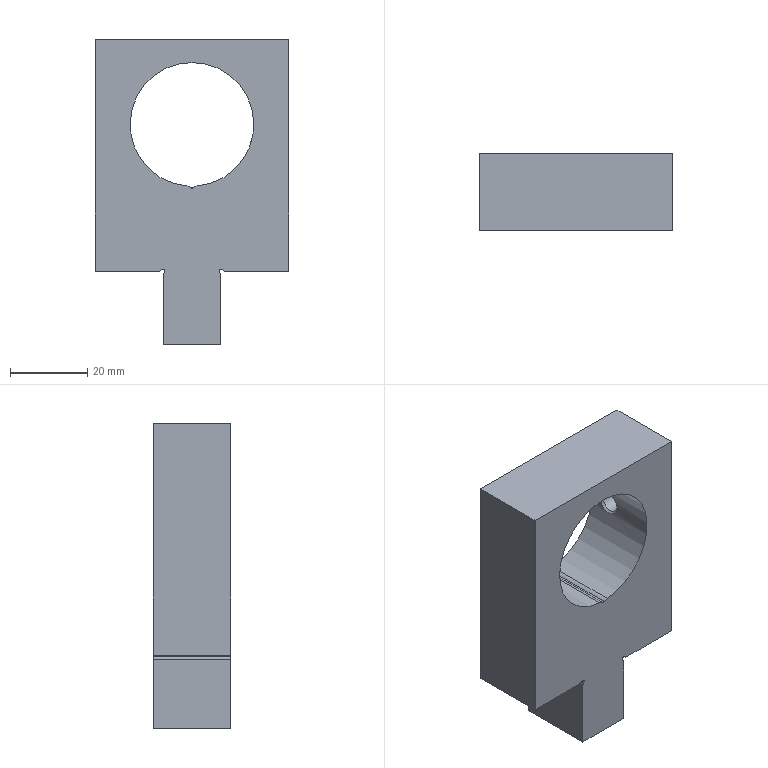Part | STEP file | 冲床-300配套压波_id890_x_t | 1 solid | 23 faces | box 50 x 20 x 79 mm | volume 49384 mm3 | cylinder 11 | plane 10 | spline 1 | cone 1 | commonest cylinder face diameters 2 x4 1 x3 4 x2 5 x1 32.01 x1
STEP:
#1=CARTESIAN_POINT('',(1916.413,80.,42.057));
#2=VERTEX_POINT('',#1);
#3=CARTESIAN_POINT('',(1913.587,80.,42.057));
#4=VERTEX_POINT('',#3);
#5=CARTESIAN_POINT('',(1915.,80.,58.));
#6=DIRECTION('',(0.,-1.,0.));
#7=DIRECTION('',(0.,0.,1.));
#8=AXIS2_PLACEMENT_3D('',#5,#6,#7);
#9=CIRCLE('',#8,16.005);
#10=EDGE_CURVE('',#2,#4,#9,.T.);
#11=ORIENTED_EDGE('',*,*,#10,.F.);
#12=CARTESIAN_POINT('',(1915.318,80.,41.609));
#13=VERTEX_POINT('',#12);
#14=CARTESIAN_POINT('',(1916.589,80.,40.065));
#15=DIRECTION('',(0.,-1.,0.));
#16=DIRECTION('',(0.,0.,1.));
#17=AXIS2_PLACEMENT_3D('',#14,#15,#16);
#18=CIRCLE('',#17,2.);
#19=EDGE_CURVE('',#2,#13,#18,.T.);
#20=ORIENTED_EDGE('',*,*,#19,.T.);
#21=CARTESIAN_POINT('',(1914.682,80.,41.609));
#22=VERTEX_POINT('',#21);
#23=CARTESIAN_POINT('',(1915.,80.,41.995));
#24=DIRECTION('',(0.,-1.,0.));
#25=DIRECTION('',(1.,0.,0.));
#26=AXIS2_PLACEMENT_3D('',#23,#24,#25);
#27=CIRCLE('',#26,0.5);
#28=EDGE_CURVE('',#22,#13,#27,.T.);
#29=ORIENTED_EDGE('',*,*,#28,.F.);
#30=CARTESIAN_POINT('',(1913.411,80.,40.065));
#31=DIRECTION('',(0.,-1.,0.));
#32=DIRECTION('',(0.,0.,1.));
#33=AXIS2_PLACEMENT_3D('',#30,#31,#32);
#34=CIRCLE('',#33,2.);
#35=EDGE_CURVE('',#22,#4,#34,.T.);
#36=ORIENTED_EDGE('',*,*,#35,.T.);
#37=EDGE_LOOP('',(#11,#20,#29,#36));
#38=FACE_BOUND('',#37,.T.);
#39=CARTESIAN_POINT('',(1890.,80.,80.));
#40=VERTEX_POINT('',#39);
#41=CARTESIAN_POINT('',(1940.,80.,80.));
#42=VERTEX_POINT('',#41);
#43=CARTESIAN_POINT('',(1940.,80.,80.));
#44=DIRECTION('',(1.,0.,0.));
#45=VECTOR('',#44,1.);
#46=LINE('',#43,#45);
#47=EDGE_CURVE('',#40,#42,#46,.T.);
#48=ORIENTED_EDGE('',*,*,#47,.F.);
#49=CARTESIAN_POINT('',(1890.,80.,20.));
#50=VERTEX_POINT('',#49);
#51=CARTESIAN_POINT('',(1890.,80.,20.));
#52=DIRECTION('',(0.,0.,1.));
#53=VECTOR('',#52,1.);
#54=LINE('',#51,#53);
#55=EDGE_CURVE('',#50,#40,#54,.T.);
#56=ORIENTED_EDGE('',*,*,#55,.F.);
#57=CARTESIAN_POINT('',(1906.382,80.,20.));
#58=VERTEX_POINT('',#57);
#59=CARTESIAN_POINT('',(1940.,80.,20.));
#60=DIRECTION('',(1.,0.,0.));
#61=VECTOR('',#60,1.);
#62=LINE('',#59,#61);
#63=EDGE_CURVE('',#50,#58,#62,.T.);
#64=ORIENTED_EDGE('',*,*,#63,.T.);
#65=CARTESIAN_POINT('',(1907.127,80.,20.333));
#66=VERTEX_POINT('',#65);
#67=CARTESIAN_POINT('',(1906.382,80.,21.));
#68=DIRECTION('',(0.,-1.,0.));
#69=DIRECTION('',(0.,0.,-1.));
#70=AXIS2_PLACEMENT_3D('',#67,#68,#69);
#71=CIRCLE('',#70,1.);
#72=EDGE_CURVE('',#58,#66,#71,.T.);
#73=ORIENTED_EDGE('',*,*,#72,.T.);
#74=CARTESIAN_POINT('',(1907.833,80.,19.627));
#75=VERTEX_POINT('',#74);
#76=CARTESIAN_POINT('',(1907.5,80.,20.));
#77=DIRECTION('',(0.,-1.,0.));
#78=DIRECTION('',(-1.,0.,0.));
#79=AXIS2_PLACEMENT_3D('',#76,#77,#78);
#80=CIRCLE('',#79,0.5);
#81=EDGE_CURVE('',#75,#66,#80,.T.);
#82=ORIENTED_EDGE('',*,*,#81,.F.);
#83=CARTESIAN_POINT('',(1907.5,80.,18.882));
#84=VERTEX_POINT('',#83);
#85=CARTESIAN_POINT('',(1908.5,80.,18.882));
#86=DIRECTION('',(0.,-1.,0.));
#87=DIRECTION('',(0.,0.,-1.));
#88=AXIS2_PLACEMENT_3D('',#85,#86,#87);
#89=CIRCLE('',#88,1.);
#90=EDGE_CURVE('',#75,#84,#89,.T.);
#91=ORIENTED_EDGE('',*,*,#90,.T.);
#92=CARTESIAN_POINT('',(1907.5,80.,1.));
#93=VERTEX_POINT('',#92);
#94=CARTESIAN_POINT('',(1907.5,80.,20.));
#95=DIRECTION('',(0.,0.,-1.));
#96=VECTOR('',#95,1.);
#97=LINE('',#94,#96);
#98=EDGE_CURVE('',#84,#93,#97,.T.);
#99=ORIENTED_EDGE('',*,*,#98,.T.);
#100=CARTESIAN_POINT('',(1922.5,80.,1.));
#101=VERTEX_POINT('',#100);
#102=CARTESIAN_POINT('',(1940.,80.,1.));
#103=DIRECTION('',(1.,0.,0.));
#104=VECTOR('',#103,1.);
#105=LINE('',#102,#104);
#106=EDGE_CURVE('',#93,#101,#105,.T.);
#107=ORIENTED_EDGE('',*,*,#106,.T.);
#108=CARTESIAN_POINT('',(1922.5,80.,18.882));
#109=VERTEX_POINT('',#108);
#110=CARTESIAN_POINT('',(1922.5,80.,-62.5));
#111=DIRECTION('',(0.,0.,1.));
#112=VECTOR('',#111,1.);
#113=LINE('',#110,#112);
#114=EDGE_CURVE('',#101,#109,#113,.T.);
#115=ORIENTED_EDGE('',*,*,#114,.T.);
#116=CARTESIAN_POINT('',(1922.167,80.,19.627));
#117=VERTEX_POINT('',#116);
#118=CARTESIAN_POINT('',(1921.5,80.,18.882));
#119=DIRECTION('',(0.,-1.,0.));
#120=DIRECTION('',(0.,0.,-1.));
#121=AXIS2_PLACEMENT_3D('',#118,#119,#120);
#122=CIRCLE('',#121,1.);
#123=EDGE_CURVE('',#109,#117,#122,.T.);
#124=ORIENTED_EDGE('',*,*,#123,.T.);
#125=CARTESIAN_POINT('',(1922.873,80.,20.333));
#126=VERTEX_POINT('',#125);
#127=CARTESIAN_POINT('',(1922.5,80.,20.));
#128=DIRECTION('',(0.,-1.,0.));
#129=DIRECTION('',(1.,0.,0.));
#130=AXIS2_PLACEMENT_3D('',#127,#128,#129);
#131=CIRCLE('',#130,0.5);
#132=EDGE_CURVE('',#126,#117,#131,.T.);
#133=ORIENTED_EDGE('',*,*,#132,.F.);
#134=CARTESIAN_POINT('',(1923.618,80.,20.));
#135=VERTEX_POINT('',#134);
#136=CARTESIAN_POINT('',(1923.618,80.,21.));
#137=DIRECTION('',(0.,-1.,0.));
#138=DIRECTION('',(0.,0.,-1.));
#139=AXIS2_PLACEMENT_3D('',#136,#137,#138);
#140=CIRCLE('',#139,1.);
#141=EDGE_CURVE('',#126,#135,#140,.T.);
#142=ORIENTED_EDGE('',*,*,#141,.T.);
#143=CARTESIAN_POINT('',(1940.,80.,20.));
#144=VERTEX_POINT('',#143);
#145=CARTESIAN_POINT('',(1940.,80.,20.));
#146=DIRECTION('',(1.,0.,0.));
#147=VECTOR('',#146,1.);
#148=LINE('',#145,#147);
#149=EDGE_CURVE('',#135,#144,#148,.T.);
#150=ORIENTED_EDGE('',*,*,#149,.T.);
#151=CARTESIAN_POINT('',(1940.,80.,20.));
#152=DIRECTION('',(0.,0.,1.));
#153=VECTOR('',#152,1.);
#154=LINE('',#151,#153);
#155=EDGE_CURVE('',#144,#42,#154,.T.);
#156=ORIENTED_EDGE('',*,*,#155,.T.);
#157=EDGE_LOOP('',(#48,#56,#64,#73,#82,#91,#99,#107,#115,#124,#133,#142,#150,#156));
#158=FACE_BOUND('',#157,.T.);
#159=CARTESIAN_POINT('',(1940.,80.,20.));
#160=DIRECTION('',(0.,1.,0.));
#161=DIRECTION('',(0.,0.,-1.));
#162=AXIS2_PLACEMENT_3D('',#159,#160,#161);
#163=PLANE('',#162);
#164=ADVANCED_FACE('',(#38,#158),#163,.F.);
#165=CARTESIAN_POINT('',(1915.318,100.,41.609));
#166=VERTEX_POINT('',#165);
#167=CARTESIAN_POINT('',(1914.682,100.,41.609));
#168=VERTEX_POINT('',#167);
#169=CARTESIAN_POINT('',(1915.,100.,41.995));
#170=DIRECTION('',(0.,1.,0.));
#171=DIRECTION('',(1.,0.,0.));
#172=AXIS2_PLACEMENT_3D('',#169,#170,#171);
#173=CIRCLE('',#172,0.5);
#174=EDGE_CURVE('',#166,#168,#173,.T.);
#175=ORIENTED_EDGE('',*,*,#174,.F.);
#176=CARTESIAN_POINT('',(1916.413,100.,42.057));
#177=VERTEX_POINT('',#176);
#178=CARTESIAN_POINT('',(1916.589,100.,40.065));
#179=DIRECTION('',(0.,1.,0.));
#180=DIRECTION('',(0.,0.,-1.));
#181=AXIS2_PLACEMENT_3D('',#178,#179,#180);
#182=CIRCLE('',#181,2.);
#183=EDGE_CURVE('',#166,#177,#182,.T.);
#184=ORIENTED_EDGE('',*,*,#183,.T.);
#185=CARTESIAN_POINT('',(1913.587,100.,42.057));
#186=VERTEX_POINT('',#185);
#187=CARTESIAN_POINT('',(1915.,100.,58.));
#188=DIRECTION('',(0.,1.,0.));
#189=DIRECTION('',(0.,0.,-1.));
#190=AXIS2_PLACEMENT_3D('',#187,#188,#189);
#191=CIRCLE('',#190,16.005);
#192=EDGE_CURVE('',#186,#177,#191,.T.);
#193=ORIENTED_EDGE('',*,*,#192,.F.);
#194=CARTESIAN_POINT('',(1913.411,100.,40.065));
#195=DIRECTION('',(0.,1.,0.));
#196=DIRECTION('',(0.,0.,-1.));
#197=AXIS2_PLACEMENT_3D('',#194,#195,#196);
#198=CIRCLE('',#197,2.);
#199=EDGE_CURVE('',#186,#168,#198,.T.);
#200=ORIENTED_EDGE('',*,*,#199,.T.);
#201=EDGE_LOOP('',(#175,#184,#193,#200));
#202=FACE_BOUND('',#201,.T.);
#203=CARTESIAN_POINT('',(1940.,100.,80.));
#204=VERTEX_POINT('',#203);
#205=CARTESIAN_POINT('',(1890.,100.,80.));
#206=VERTEX_POINT('',#205);
#207=CARTESIAN_POINT('',(1940.,100.,80.));
#208=DIRECTION('',(-1.,0.,0.));
#209=VECTOR('',#208,1.);
#210=LINE('',#207,#209);
#211=EDGE_CURVE('',#204,#206,#210,.T.);
#212=ORIENTED_EDGE('',*,*,#211,.F.);
#213=CARTESIAN_POINT('',(1940.,100.,20.));
#214=VERTEX_POINT('',#213);
#215=CARTESIAN_POINT('',(1940.,100.,20.));
#216=DIRECTION('',(0.,0.,-1.));
#217=VECTOR('',#216,1.);
#218=LINE('',#215,#217);
#219=EDGE_CURVE('',#204,#214,#218,.T.);
#220=ORIENTED_EDGE('',*,*,#219,.T.);
#221=CARTESIAN_POINT('',(1923.618,100.,20.));
#222=VERTEX_POINT('',#221);
#223=CARTESIAN_POINT('',(1940.,100.,20.));
#224=DIRECTION('',(-1.,0.,0.));
#225=VECTOR('',#224,1.);
#226=LINE('',#223,#225);
#227=EDGE_CURVE('',#214,#222,#226,.T.);
#228=ORIENTED_EDGE('',*,*,#227,.T.);
#229=CARTESIAN_POINT('',(1922.873,100.,20.333));
#230=VERTEX_POINT('',#229);
#231=CARTESIAN_POINT('',(1923.618,100.,21.));
#232=DIRECTION('',(0.,1.,0.));
#233=DIRECTION('',(0.,0.,1.));
#234=AXIS2_PLACEMENT_3D('',#231,#232,#233);
#235=CIRCLE('',#234,1.);
#236=EDGE_CURVE('',#222,#230,#235,.T.);
#237=ORIENTED_EDGE('',*,*,#236,.T.);
#238=CARTESIAN_POINT('',(1922.167,100.,19.627));
#239=VERTEX_POINT('',#238);
#240=CARTESIAN_POINT('',(1922.5,100.,20.));
#241=DIRECTION('',(0.,1.,0.));
#242=DIRECTION('',(1.,0.,0.));
#243=AXIS2_PLACEMENT_3D('',#240,#241,#242);
#244=CIRCLE('',#243,0.5);
#245=EDGE_CURVE('',#239,#230,#244,.T.);
#246=ORIENTED_EDGE('',*,*,#245,.F.);
#247=CARTESIAN_POINT('',(1922.5,100.,18.882));
#248=VERTEX_POINT('',#247);
#249=CARTESIAN_POINT('',(1921.5,100.,18.882));
#250=DIRECTION('',(0.,1.,0.));
#251=DIRECTION('',(0.,0.,1.));
#252=AXIS2_PLACEMENT_3D('',#249,#250,#251);
#253=CIRCLE('',#252,1.);
#254=EDGE_CURVE('',#239,#248,#253,.T.);
#255=ORIENTED_EDGE('',*,*,#254,.T.);
#256=CARTESIAN_POINT('',(1922.5,100.,1.));
#257=VERTEX_POINT('',#256);
#258=CARTESIAN_POINT('',(1922.5,100.,20.));
#259=DIRECTION('',(0.,0.,-1.));
#260=VECTOR('',#259,1.);
#261=LINE('',#258,#260);
#262=EDGE_CURVE('',#248,#257,#261,.T.);
#263=ORIENTED_EDGE('',*,*,#262,.T.);
#264=CARTESIAN_POINT('',(1907.5,100.,1.));
#265=VERTEX_POINT('',#264);
#266=CARTESIAN_POINT('',(1940.,100.,1.));
#267=DIRECTION('',(-1.,0.,0.));
#268=VECTOR('',#267,1.);
#269=LINE('',#266,#268);
#270=EDGE_CURVE('',#257,#265,#269,.T.);
#271=ORIENTED_EDGE('',*,*,#270,.T.);
#272=CARTESIAN_POINT('',(1907.5,100.,18.882));
#273=VERTEX_POINT('',#272);
#274=CARTESIAN_POINT('',(1907.5,100.,-62.5));
#275=DIRECTION('',(0.,0.,1.));
#276=VECTOR('',#275,1.);
#277=LINE('',#274,#276);
#278=EDGE_CURVE('',#265,#273,#277,.T.);
#279=ORIENTED_EDGE('',*,*,#278,.T.);
#280=CARTESIAN_POINT('',(1907.833,100.,19.627));
#281=VERTEX_POINT('',#280);
#282=CARTESIAN_POINT('',(1908.5,100.,18.882));
#283=DIRECTION('',(0.,1.,0.));
#284=DIRECTION('',(0.,0.,1.));
#285=AXIS2_PLACEMENT_3D('',#282,#283,#284);
#286=CIRCLE('',#285,1.);
#287=EDGE_CURVE('',#273,#281,#286,.T.);
#288=ORIENTED_EDGE('',*,*,#287,.T.);
#289=CARTESIAN_POINT('',(1907.127,100.,20.333));
#290=VERTEX_POINT('',#289);
#291=CARTESIAN_POINT('',(1907.5,100.,20.));
#292=DIRECTION('',(0.,1.,0.));
#293=DIRECTION('',(-1.,0.,0.));
#294=AXIS2_PLACEMENT_3D('',#291,#292,#293);
#295=CIRCLE('',#294,0.5);
#296=EDGE_CURVE('',#290,#281,#295,.T.);
#297=ORIENTED_EDGE('',*,*,#296,.F.);
#298=CARTESIAN_POINT('',(1906.382,100.,20.));
#299=VERTEX_POINT('',#298);
#300=CARTESIAN_POINT('',(1906.382,100.,21.));
#301=DIRECTION('',(0.,1.,0.));
#302=DIRECTION('',(0.,0.,1.));
#303=AXIS2_PLACEMENT_3D('',#300,#301,#302);
#304=CIRCLE('',#303,1.);
#305=EDGE_CURVE('',#290,#299,#304,.T.);
#306=ORIENTED_EDGE('',*,*,#305,.T.);
#307=CARTESIAN_POINT('',(1890.,100.,20.));
#308=VERTEX_POINT('',#307);
#309=CARTESIAN_POINT('',(1940.,100.,20.));
#310=DIRECTION('',(-1.,0.,0.));
#311=VECTOR('',#310,1.);
#312=LINE('',#309,#311);
#313=EDGE_CURVE('',#299,#308,#312,.T.);
#314=ORIENTED_EDGE('',*,*,#313,.T.);
#315=CARTESIAN_POINT('',(1890.,100.,20.));
#316=DIRECTION('',(0.,0.,-1.));
#317=VECTOR('',#316,1.);
#318=LINE('',#315,#317);
#319=EDGE_CURVE('',#206,#308,#318,.T.);
#320=ORIENTED_EDGE('',*,*,#319,.F.);
#321=EDGE_LOOP('',(#212,#220,#228,#237,#246,#255,#263,#271,#279,#288,#297,#306,#314,#320));
#322=FACE_BOUND('',#321,.T.);
#323=CARTESIAN_POINT('',(1940.,100.,20.));
#324=DIRECTION('',(0.,-1.,0.));
#325=DIRECTION('',(0.,0.,1.));
#326=AXIS2_PLACEMENT_3D('',#323,#324,#325);
#327=PLANE('',#326);
#328=ADVANCED_FACE('',(#202,#322),#327,.F.);
#329=CARTESIAN_POINT('',(1890.,80.,80.));
#330=DIRECTION('',(0.,-1.,0.));
#331=VECTOR('',#330,1.);
#332=LINE('',#329,#331);
#333=EDGE_CURVE('',#206,#40,#332,.T.);
#334=ORIENTED_EDGE('',*,*,#333,.F.);
#335=ORIENTED_EDGE('',*,*,#319,.T.);
#336=CARTESIAN_POINT('',(1890.,-80.,20.));
#337=DIRECTION('',(0.,-1.,0.));
#338=VECTOR('',#337,1.);
#339=LINE('',#336,#338);
#340=EDGE_CURVE('',#308,#50,#339,.T.);
#341=ORIENTED_EDGE('',*,*,#340,.T.);
#342=ORIENTED_EDGE('',*,*,#55,.T.);
#343=EDGE_LOOP('',(#334,#335,#341,#342));
#344=FACE_OUTER_BOUND('',#343,.T.);
#345=CARTESIAN_POINT('',(1890.,80.,20.));
#346=DIRECTION('',(1.,0.,0.));
#347=DIRECTION('',(0.,0.,-1.));
#348=AXIS2_PLACEMENT_3D('',#345,#346,#347);
#349=PLANE('',#348);
#350=ADVANCED_FACE('',(#344),#349,.F.);
#351=CARTESIAN_POINT('',(1940.,94.,61.));
#352=VERTEX_POINT('',#351);
#353=CARTESIAN_POINT('',(1940.,94.,58.));
#354=DIRECTION('',(-1.,0.,0.));
#355=DIRECTION('',(0.,0.,1.));
#356=AXIS2_PLACEMENT_3D('',#353,#354,#355);
#357=CIRCLE('',#356,3.);
#358=EDGE_CURVE('',#352,#352,#357,.T.);
#359=ORIENTED_EDGE('',*,*,#358,.T.);
#360=EDGE_LOOP('',(#359));
#361=FACE_BOUND('',#360,.T.);
#362=CARTESIAN_POINT('',(1940.,150.,80.));
#363=DIRECTION('',(0.,1.,0.));
#364=VECTOR('',#363,1.);
#365=LINE('',#362,#364);
#366=EDGE_CURVE('',#42,#204,#365,.T.);
#367=ORIENTED_EDGE('',*,*,#366,.F.);
#368=ORIENTED_EDGE('',*,*,#155,.F.);
#369=CARTESIAN_POINT('',(1940.,-150.,20.));
#370=DIRECTION('',(0.,1.,0.));
#371=VECTOR('',#370,1.);
#372=LINE('',#369,#371);
#373=EDGE_CURVE('',#144,#214,#372,.T.);
#374=ORIENTED_EDGE('',*,*,#373,.T.);
#375=ORIENTED_EDGE('',*,*,#219,.F.);
#376=EDGE_LOOP('',(#367,#368,#374,#375));
#377=FACE_BOUND('',#376,.T.);
#378=CARTESIAN_POINT('',(1940.,150.,20.));
#379=DIRECTION('',(-1.,0.,0.));
#380=DIRECTION('',(0.,0.,1.));
#381=AXIS2_PLACEMENT_3D('',#378,#379,#380);
#382=PLANE('',#381);
#383=ADVANCED_FACE('',(#361,#377),#382,.F.);
#384=ORIENTED_EDGE('',*,*,#28,.T.);
#385=CARTESIAN_POINT('',(1915.318,80.,41.609));
#386=DIRECTION('',(0.,1.,0.));
#387=VECTOR('',#386,1.);
#388=LINE('',#385,#387);
#389=EDGE_CURVE('',#13,#166,#388,.T.);
#390=ORIENTED_EDGE('',*,*,#389,.T.);
#391=ORIENTED_EDGE('',*,*,#174,.T.);
#392=CARTESIAN_POINT('',(1914.682,80.,41.609));
#393=DIRECTION('',(0.,-1.,0.));
#394=VECTOR('',#393,1.);
#395=LINE('',#392,#394);
#396=EDGE_CURVE('',#168,#22,#395,.T.);
#397=ORIENTED_EDGE('',*,*,#396,.T.);
#398=EDGE_LOOP('',(#384,#390,#391,#397));
#399=FACE_OUTER_BOUND('',#398,.T.);
#400=CARTESIAN_POINT('',(1915.,80.,41.995));
#401=DIRECTION('',(0.,1.,0.));
#402=DIRECTION('',(0.,0.,1.));
#403=AXIS2_PLACEMENT_3D('',#400,#401,#402);
#404=CYLINDRICAL_SURFACE('',#403,0.5);
#405=ADVANCED_FACE('',(#399),#404,.F.);
#406=ORIENTED_EDGE('',*,*,#183,.F.);
#407=ORIENTED_EDGE('',*,*,#389,.F.);
#408=ORIENTED_EDGE('',*,*,#19,.F.);
#409=CARTESIAN_POINT('',(1916.413,105.,42.057));
#410=DIRECTION('',(0.,-1.,0.));
#411=VECTOR('',#410,1.);
#412=LINE('',#409,#411);
#413=EDGE_CURVE('',#177,#2,#412,.T.);
#414=ORIENTED_EDGE('',*,*,#413,.F.);
#415=EDGE_LOOP('',(#406,#407,#408,#414));
#416=FACE_OUTER_BOUND('',#415,.T.);
#417=CARTESIAN_POINT('',(1916.589,80.,40.065));
#418=DIRECTION('',(0.,-1.,0.));
#419=DIRECTION('',(0.,0.,-1.));
#420=AXIS2_PLACEMENT_3D('',#417,#418,#419);
#421=CYLINDRICAL_SURFACE('',#420,2.);
#422=ADVANCED_FACE('',(#416),#421,.T.);
#423=CARTESIAN_POINT('',(1931.303,94.,60.5));
#424=VERTEX_POINT('',#423);
#425=CARTESIAN_POINT('',(1931.303,94.,60.5));
#426=CARTESIAN_POINT('',(1931.303,94.488,60.5));
#427=CARTESIAN_POINT('',(1931.351,95.187,60.349));
#428=CARTESIAN_POINT('',(1931.445,95.768,59.768));
#429=CARTESIAN_POINT('',(1931.539,96.349,59.187));
#430=CARTESIAN_POINT('',(1931.585,96.5,58.495));
#431=CARTESIAN_POINT('',(1931.585,96.5,58.001));
#432=CARTESIAN_POINT('',(1931.585,96.5,57.508));
#433=CARTESIAN_POINT('',(1931.538,96.344,56.809));
#434=CARTESIAN_POINT('',(1931.445,95.768,56.233));
#435=CARTESIAN_POINT('',(1931.351,95.192,55.656));
#436=CARTESIAN_POINT('',(1931.303,94.486,55.5));
#437=CARTESIAN_POINT('',(1931.303,94.,55.5));
#438=CARTESIAN_POINT('',(1931.303,93.513,55.5));
#439=CARTESIAN_POINT('',(1931.351,92.813,55.651));
#440=CARTESIAN_POINT('',(1931.445,92.231,56.233));
#441=CARTESIAN_POINT('',(1931.539,91.65,56.815));
#442=CARTESIAN_POINT('',(1931.585,91.5,57.507));
#443=CARTESIAN_POINT('',(1931.585,91.5,58.001));
#444=CARTESIAN_POINT('',(1931.585,91.5,58.496));
#445=CARTESIAN_POINT('',(1931.538,91.656,59.192));
#446=CARTESIAN_POINT('',(1931.445,92.232,59.768));
#447=CARTESIAN_POINT('',(1931.351,92.808,60.343));
#448=CARTESIAN_POINT('',(1931.303,93.512,60.5));
#449=CARTESIAN_POINT('',(1931.303,94.,60.5));
#450=B_SPLINE_CURVE_WITH_KNOTS('',3,(#425,#426,#427,#428,#429,#430,#431,#432,#433,#434,#435,#436,#437,#438,#439,#440,#441,#442,#443,#444,#445,#446,#447,#448,#449),.UNSPECIFIED.,.T.,.F.,(1,3,3,3,3,3,3,3,3,3,1),(-0.125,0.,0.125,0.25,0.375,0.5,0.625,0.75,0.875,1.,1.125),.UNSPECIFIED.);
#451=EDGE_CURVE('',#424,#424,#450,.T.);
#452=ORIENTED_EDGE('',*,*,#451,.T.);
#453=EDGE_LOOP('',(#452));
#454=FACE_BOUND('',#453,.T.);
#455=CARTESIAN_POINT('',(1939.5,94.,60.5));
#456=VERTEX_POINT('',#455);
#457=CARTESIAN_POINT('',(1939.5,94.,58.));
#458=DIRECTION('',(1.,0.,0.));
#459=DIRECTION('',(0.,0.,1.));
#460=AXIS2_PLACEMENT_3D('',#457,#458,#459);
#461=CIRCLE('',#460,2.5);
#462=EDGE_CURVE('',#456,#456,#461,.T.);
#463=ORIENTED_EDGE('',*,*,#462,.T.);
#464=EDGE_LOOP('',(#463));
#465=FACE_BOUND('',#464,.T.);
#466=CARTESIAN_POINT('',(1940.,94.,58.));
#467=DIRECTION('',(-1.,0.,0.));
#468=DIRECTION('',(0.,0.,1.));
#469=AXIS2_PLACEMENT_3D('',#466,#467,#468);
#470=CYLINDRICAL_SURFACE('',#469,2.5);
#471=ADVANCED_FACE('',(#454,#465),#470,.F.);
#472=CARTESIAN_POINT('',(1930.734,94.,55.068));
#473=VERTEX_POINT('',#472);
#474=CARTESIAN_POINT('',(1930.734,94.,55.068));
#475=CARTESIAN_POINT('',(1930.734,94.344,55.068));
#476=CARTESIAN_POINT('',(1930.745,94.693,55.127));
#477=CARTESIAN_POINT('',(1930.765,95.018,55.238));
#478=CARTESIAN_POINT('',(1930.785,95.343,55.35));
#479=CARTESIAN_POINT('',(1930.813,95.654,55.519));
#480=CARTESIAN_POINT('',(1930.843,95.924,55.731));
#481=CARTESIAN_POINT('',(1930.874,96.197,55.945));
#482=CARTESIAN_POINT('',(1930.908,96.434,56.212));
#483=CARTESIAN_POINT('',(1930.935,96.614,56.509));
#484=CARTESIAN_POINT('',(1930.962,96.783,56.788));
#485=CARTESIAN_POINT('',(1930.983,96.908,57.1));
#486=CARTESIAN_POINT('',(1930.994,96.977,57.42));
#487=CARTESIAN_POINT('',(1931.006,97.046,57.742));
#488=CARTESIAN_POINT('',(1931.008,97.058,58.082));
#489=CARTESIAN_POINT('',(1931.,97.009,58.408));
#490=CARTESIAN_POINT('',(1930.992,96.964,58.709));
#491=CARTESIAN_POINT('',(1930.976,96.869,59.005));
#492=CARTESIAN_POINT('',(1930.954,96.733,59.277));
#493=CARTESIAN_POINT('',(1930.931,96.589,59.565));
#494=CARTESIAN_POINT('',(1930.901,96.395,59.833));
#495=CARTESIAN_POINT('',(1930.872,96.165,60.058));
#496=CARTESIAN_POINT('',(1930.843,95.933,60.285));
#497=CARTESIAN_POINT('',(1930.813,95.659,60.475));
#498=CARTESIAN_POINT('',(1930.79,95.366,60.617));
#499=CARTESIAN_POINT('',(1930.765,95.059,60.766));
#500=CARTESIAN_POINT('',(1930.746,94.722,60.866));
#501=CARTESIAN_POINT('',(1930.739,94.383,60.908));
#502=CARTESIAN_POINT('',(1930.737,94.297,60.919));
#503=CARTESIAN_POINT('',(1930.735,94.211,60.926));
#504=CARTESIAN_POINT('',(1930.735,94.125,60.93));
#505=CARTESIAN_POINT('',(1930.734,94.039,60.933));
#506=CARTESIAN_POINT('',(1930.734,93.953,60.933));
#507=CARTESIAN_POINT('',(1930.735,93.867,60.929));
#508=CARTESIAN_POINT('',(1930.737,93.524,60.914));
#509=CARTESIAN_POINT('',(1930.751,93.179,60.841));
#510=CARTESIAN_POINT('',(1930.773,92.86,60.716));
#511=CARTESIAN_POINT('',(1930.794,92.541,60.591));
#512=CARTESIAN_POINT('',(1930.824,92.239,60.412));
#513=CARTESIAN_POINT('',(1930.854,91.979,60.19));
#514=CARTESIAN_POINT('',(1930.886,91.715,59.965));
#515=CARTESIAN_POINT('',(1930.919,91.49,59.687));
#516=CARTESIAN_POINT('',(1930.945,91.323,59.383));
#517=CARTESIAN_POINT('',(1930.97,91.166,59.098));
#518=CARTESIAN_POINT('',(1930.989,91.054,58.782));
#519=CARTESIAN_POINT('',(1930.998,90.999,58.461));
#520=CARTESIAN_POINT('',(1931.008,90.945,58.139));
#521=CARTESIAN_POINT('',(1931.007,90.949,57.802));
#522=CARTESIAN_POINT('',(1930.997,91.01,57.482));
#523=CARTESIAN_POINT('',(1930.987,91.067,57.184));
#524=CARTESIAN_POINT('',(1930.969,91.173,56.892));
#525=CARTESIAN_POINT('',(1930.946,91.318,56.626));
#526=CARTESIAN_POINT('',(1930.921,91.474,56.34));
#527=CARTESIAN_POINT('',(1930.891,91.681,56.077));
#528=CARTESIAN_POINT('',(1930.861,91.923,55.859));
#529=CARTESIAN_POINT('',(1930.832,92.165,55.642));
#530=CARTESIAN_POINT('',(1930.803,92.445,55.463));
#531=CARTESIAN_POINT('',(1930.781,92.742,55.332));
#532=CARTESIAN_POINT('',(1930.758,93.057,55.194));
#533=CARTESIAN_POINT('',(1930.741,93.4,55.107));
#534=CARTESIAN_POINT('',(1930.736,93.744,55.078));
#535=CARTESIAN_POINT('',(1930.735,93.829,55.071));
#536=CARTESIAN_POINT('',(1930.734,93.914,55.068));
#537=CARTESIAN_POINT('',(1930.734,94.,55.068));
#538=B_SPLINE_CURVE_WITH_KNOTS('',3,(#474,#475,#476,#477,#478,#479,#480,#481,#482,#483,#484,#485,#486,#487,#488,#489,#490,#491,#492,#493,#494,#495,#496,#497,#498,#499,#500,#501,#502,#503,#504,#505,#506,#507,#508,#509,#510,#511,#512,#513,#514,#515,#516,#517,#518,#519,#520,#521,#522,#523,#524,#525,#526,#527,#528,#529,#530,#531,#532,#533,#534,#535,#536,#537),.UNSPECIFIED.,.T.,.F.,(1,3,3,3,3,3,3,3,3,3,3,3,3,3,3,3,3,3,3,3,3,3,3,1),(-0.01354,0.,0.05524,0.1106,0.1666,0.2191,0.2721,0.3208,0.3727,0.4249,0.4798,0.4934,0.5071,0.5622,0.6172,0.6731,0.7255,0.7779,0.8265,0.879,0.9312,0.9865,1.,1.055),.UNSPECIFIED.);
#539=EDGE_CURVE('',#473,#473,#538,.T.);
#540=ORIENTED_EDGE('',*,*,#539,.F.);
#541=EDGE_LOOP('',(#540));
#542=FACE_BOUND('',#541,.T.);
#543=ORIENTED_EDGE('',*,*,#451,.F.);
#544=EDGE_LOOP('',(#543));
#545=FACE_BOUND('',#544,.T.);
#546=CARTESIAN_POINT('',(1931.303,94.657,60.5));
#547=CARTESIAN_POINT('',(1931.303,93.343,60.5));
#548=CARTESIAN_POINT('',(1931.37,92.694,60.229));
#549=CARTESIAN_POINT('',(1931.52,91.77,59.306));
#550=CARTESIAN_POINT('',(1931.585,91.5,58.658));
#551=CARTESIAN_POINT('',(1931.585,91.5,57.344));
#552=CARTESIAN_POINT('',(1931.52,91.769,56.696));
#553=CARTESIAN_POINT('',(1931.37,92.694,55.77));
#554=CARTESIAN_POINT('',(1931.303,93.34,55.5));
#555=CARTESIAN_POINT('',(1931.303,94.66,55.5));
#556=CARTESIAN_POINT('',(1931.37,95.306,55.77));
#557=CARTESIAN_POINT('',(1931.52,96.231,56.695));
#558=CARTESIAN_POINT('',(1931.585,96.5,57.345));
#559=CARTESIAN_POINT('',(1931.585,96.5,58.658));
#560=CARTESIAN_POINT('',(1931.52,96.23,59.306));
#561=CARTESIAN_POINT('',(1931.37,95.306,60.229));
#562=CARTESIAN_POINT('',(1931.303,94.657,60.5));
#563=CARTESIAN_POINT('',(1931.303,93.343,60.5));
#564=CARTESIAN_POINT('',(1930.728,94.801,60.937));
#565=CARTESIAN_POINT('',(1930.728,93.199,60.937));
#566=CARTESIAN_POINT('',(1930.792,92.41,60.619));
#567=CARTESIAN_POINT('',(1930.937,91.284,59.534));
#568=CARTESIAN_POINT('',(1931.,90.956,58.773));
#569=CARTESIAN_POINT('',(1931.,90.956,57.23));
#570=CARTESIAN_POINT('',(1930.937,91.283,56.468));
#571=CARTESIAN_POINT('',(1930.792,92.41,55.381));
#572=CARTESIAN_POINT('',(1930.728,93.196,55.063));
#573=CARTESIAN_POINT('',(1930.728,94.804,55.063));
#574=CARTESIAN_POINT('',(1930.792,95.59,55.38));
#575=CARTESIAN_POINT('',(1930.937,96.716,56.467));
#576=CARTESIAN_POINT('',(1931.,97.044,57.23));
#577=CARTESIAN_POINT('',(1931.,97.044,58.773));
#578=CARTESIAN_POINT('',(1930.937,96.716,59.534));
#579=CARTESIAN_POINT('',(1930.792,95.59,60.619));
#580=CARTESIAN_POINT('',(1930.728,94.801,60.937));
#581=CARTESIAN_POINT('',(1930.728,93.199,60.937));
#582=B_SPLINE_SURFACE_WITH_KNOTS('',1,3,((#546,#547,#548,#549,#550,#551,#552,#553,#554,#555,#556,#557,#558,#559,#560,#561,#562,#563),(#564,#565,#566,#567,#568,#569,#570,#571,#572,#573,#574,#575,#576,#577,#578,#579,#580,#581)),.UNSPECIFIED.,.F.,.T.,.F.,(2,2),(2,2,2,2,2,2,2,2,2,2,2),(0.,1.),(-0.125,0.,0.125,0.25,0.375,0.5,0.625,0.75,0.875,1.,1.125),.UNSPECIFIED.);
#583=ADVANCED_FACE('',(#542,#545),#582,.F.);
#584=ORIENTED_EDGE('',*,*,#35,.F.);
#585=ORIENTED_EDGE('',*,*,#396,.F.);
#586=ORIENTED_EDGE('',*,*,#199,.F.);
#587=CARTESIAN_POINT('',(1913.587,105.,42.057));
#588=DIRECTION('',(0.,1.,0.));
#589=VECTOR('',#588,1.);
#590=LINE('',#587,#589);
#591=EDGE_CURVE('',#4,#186,#590,.T.);
#592=ORIENTED_EDGE('',*,*,#591,.F.);
#593=EDGE_LOOP('',(#584,#585,#586,#592));
#594=FACE_OUTER_BOUND('',#593,.T.);
#595=CARTESIAN_POINT('',(1913.411,80.,40.065));
#596=DIRECTION('',(0.,1.,0.));
#597=DIRECTION('',(0.,0.,1.));
#598=AXIS2_PLACEMENT_3D('',#595,#596,#597);
#599=CYLINDRICAL_SURFACE('',#598,2.);
#600=ADVANCED_FACE('',(#594),#599,.T.);
#601=ORIENTED_EDGE('',*,*,#539,.T.);
#602=EDGE_LOOP('',(#601));
#603=FACE_BOUND('',#602,.T.);
#604=ORIENTED_EDGE('',*,*,#192,.T.);
#605=ORIENTED_EDGE('',*,*,#413,.T.);
#606=ORIENTED_EDGE('',*,*,#10,.T.);
#607=ORIENTED_EDGE('',*,*,#591,.T.);
#608=EDGE_LOOP('',(#604,#605,#606,#607));
#609=FACE_BOUND('',#608,.T.);
#610=CARTESIAN_POINT('',(1915.,105.,58.));
#611=DIRECTION('',(0.,-1.,0.));
#612=DIRECTION('',(0.,0.,1.));
#613=AXIS2_PLACEMENT_3D('',#610,#611,#612);
#614=CYLINDRICAL_SURFACE('',#613,16.005);
#615=ADVANCED_FACE('',(#603,#609),#614,.F.);
#616=ORIENTED_EDGE('',*,*,#462,.F.);
#617=EDGE_LOOP('',(#616));
#618=FACE_BOUND('',#617,.T.);
#619=ORIENTED_EDGE('',*,*,#358,.F.);
#620=EDGE_LOOP('',(#619));
#621=FACE_BOUND('',#620,.T.);
#622=CARTESIAN_POINT('',(1940.,94.,58.));
#623=DIRECTION('',(1.,0.,0.));
#624=DIRECTION('',(0.,0.,-1.));
#625=AXIS2_PLACEMENT_3D('',#622,#623,#624);
#626=CONICAL_SURFACE('',#625,3.,45.);
#627=ADVANCED_FACE('',(#618,#621),#626,.F.);
#628=ORIENTED_EDGE('',*,*,#63,.F.);
#629=ORIENTED_EDGE('',*,*,#340,.F.);
#630=ORIENTED_EDGE('',*,*,#313,.F.);
#631=CARTESIAN_POINT('',(1906.382,100.,20.));
#632=DIRECTION('',(0.,-1.,0.));
#633=VECTOR('',#632,1.);
#634=LINE('',#631,#633);
#635=EDGE_CURVE('',#299,#58,#634,.T.);
#636=ORIENTED_EDGE('',*,*,#635,.T.);
#637=EDGE_LOOP('',(#628,#629,#630,#636));
#638=FACE_OUTER_BOUND('',#637,.T.);
#639=CARTESIAN_POINT('',(2070.,207.5,20.));
#640=DIRECTION('',(0.,0.,1.));
#641=DIRECTION('',(1.,0.,0.));
#642=AXIS2_PLACEMENT_3D('',#639,#640,#641);
#643=PLANE('',#642);
#644=ADVANCED_FACE('',(#638),#643,.F.);
#645=ORIENTED_EDGE('',*,*,#278,.F.);
#646=CARTESIAN_POINT('',(1907.5,207.5,1.));
#647=DIRECTION('',(0.,-1.,0.));
#648=VECTOR('',#647,1.);
#649=LINE('',#646,#648);
#650=EDGE_CURVE('',#265,#93,#649,.T.);
#651=ORIENTED_EDGE('',*,*,#650,.T.);
#652=ORIENTED_EDGE('',*,*,#98,.F.);
#653=CARTESIAN_POINT('',(1907.5,66.994,18.882));
#654=DIRECTION('',(0.,1.,0.));
#655=VECTOR('',#654,1.);
#656=LINE('',#653,#655);
#657=EDGE_CURVE('',#84,#273,#656,.T.);
#658=ORIENTED_EDGE('',*,*,#657,.T.);
#659=EDGE_LOOP('',(#645,#651,#652,#658));
#660=FACE_OUTER_BOUND('',#659,.T.);
#661=CARTESIAN_POINT('',(1907.5,66.994,-62.5));
#662=DIRECTION('',(-1.,0.,0.));
#663=DIRECTION('',(0.,0.,1.));
#664=AXIS2_PLACEMENT_3D('',#661,#662,#663);
#665=PLANE('',#664);
#666=ADVANCED_FACE('',(#660),#665,.T.);
#667=ORIENTED_EDGE('',*,*,#227,.F.);
#668=ORIENTED_EDGE('',*,*,#373,.F.);
#669=ORIENTED_EDGE('',*,*,#149,.F.);
#670=CARTESIAN_POINT('',(1923.618,80.,20.));
#671=DIRECTION('',(0.,1.,0.));
#672=VECTOR('',#671,1.);
#673=LINE('',#670,#672);
#674=EDGE_CURVE('',#135,#222,#673,.T.);
#675=ORIENTED_EDGE('',*,*,#674,.T.);
#676=EDGE_LOOP('',(#667,#668,#669,#675));
#677=FACE_OUTER_BOUND('',#676,.T.);
#678=CARTESIAN_POINT('',(2070.,207.5,20.));
#679=DIRECTION('',(0.,0.,1.));
#680=DIRECTION('',(1.,0.,0.));
#681=AXIS2_PLACEMENT_3D('',#678,#679,#680);
#682=PLANE('',#681);
#683=ADVANCED_FACE('',(#677),#682,.F.);
#684=ORIENTED_EDGE('',*,*,#114,.F.);
#685=CARTESIAN_POINT('',(1922.5,207.5,1.));
#686=DIRECTION('',(0.,1.,0.));
#687=VECTOR('',#686,1.);
#688=LINE('',#685,#687);
#689=EDGE_CURVE('',#101,#257,#688,.T.);
#690=ORIENTED_EDGE('',*,*,#689,.T.);
#691=ORIENTED_EDGE('',*,*,#262,.F.);
#692=CARTESIAN_POINT('',(1922.5,105.994,18.882));
#693=DIRECTION('',(0.,-1.,0.));
#694=VECTOR('',#693,1.);
#695=LINE('',#692,#694);
#696=EDGE_CURVE('',#248,#109,#695,.T.);
#697=ORIENTED_EDGE('',*,*,#696,.T.);
#698=EDGE_LOOP('',(#684,#690,#691,#697));
#699=FACE_OUTER_BOUND('',#698,.T.);
#700=CARTESIAN_POINT('',(1922.5,105.994,-62.5));
#701=DIRECTION('',(1.,0.,0.));
#702=DIRECTION('',(0.,0.,-1.));
#703=AXIS2_PLACEMENT_3D('',#700,#701,#702);
#704=PLANE('',#703);
#705=ADVANCED_FACE('',(#699),#704,.T.);
#706=ORIENTED_EDGE('',*,*,#650,.F.);
#707=ORIENTED_EDGE('',*,*,#270,.F.);
#708=ORIENTED_EDGE('',*,*,#689,.F.);
#709=ORIENTED_EDGE('',*,*,#106,.F.);
#710=EDGE_LOOP('',(#706,#707,#708,#709));
#711=FACE_OUTER_BOUND('',#710,.T.);
#712=CARTESIAN_POINT('',(2070.,207.5,1.));
#713=DIRECTION('',(0.,0.,1.));
#714=DIRECTION('',(1.,0.,0.));
#715=AXIS2_PLACEMENT_3D('',#712,#713,#714);
#716=PLANE('',#715);
#717=ADVANCED_FACE('',(#711),#716,.F.);
#718=ORIENTED_EDGE('',*,*,#245,.T.);
#719=CARTESIAN_POINT('',(1922.873,100.,20.333));
#720=DIRECTION('',(0.,-1.,0.));
#721=VECTOR('',#720,1.);
#722=LINE('',#719,#721);
#723=EDGE_CURVE('',#230,#126,#722,.T.);
#724=ORIENTED_EDGE('',*,*,#723,.T.);
#725=ORIENTED_EDGE('',*,*,#132,.T.);
#726=CARTESIAN_POINT('',(1922.167,100.,19.627));
#727=DIRECTION('',(0.,1.,0.));
#728=VECTOR('',#727,1.);
#729=LINE('',#726,#728);
#730=EDGE_CURVE('',#117,#239,#729,.T.);
#731=ORIENTED_EDGE('',*,*,#730,.T.);
#732=EDGE_LOOP('',(#718,#724,#725,#731));
#733=FACE_OUTER_BOUND('',#732,.T.);
#734=CARTESIAN_POINT('',(1922.5,100.,20.));
#735=DIRECTION('',(0.,-1.,0.));
#736=DIRECTION('',(0.,0.,1.));
#737=AXIS2_PLACEMENT_3D('',#734,#735,#736);
#738=CYLINDRICAL_SURFACE('',#737,0.5);
#739=ADVANCED_FACE('',(#733),#738,.F.);
#740=ORIENTED_EDGE('',*,*,#296,.T.);
#741=CARTESIAN_POINT('',(1907.833,80.,19.627));
#742=DIRECTION('',(0.,-1.,0.));
#743=VECTOR('',#742,1.);
#744=LINE('',#741,#743);
#745=EDGE_CURVE('',#281,#75,#744,.T.);
#746=ORIENTED_EDGE('',*,*,#745,.T.);
#747=ORIENTED_EDGE('',*,*,#81,.T.);
#748=CARTESIAN_POINT('',(1907.127,80.,20.333));
#749=DIRECTION('',(0.,1.,0.));
#750=VECTOR('',#749,1.);
#751=LINE('',#748,#750);
#752=EDGE_CURVE('',#66,#290,#751,.T.);
#753=ORIENTED_EDGE('',*,*,#752,.T.);
#754=EDGE_LOOP('',(#740,#746,#747,#753));
#755=FACE_OUTER_BOUND('',#754,.T.);
#756=CARTESIAN_POINT('',(1907.5,80.,20.));
#757=DIRECTION('',(0.,1.,0.));
#758=DIRECTION('',(0.,0.,-1.));
#759=AXIS2_PLACEMENT_3D('',#756,#757,#758);
#760=CYLINDRICAL_SURFACE('',#759,0.5);
#761=ADVANCED_FACE('',(#755),#760,.F.);
#762=ORIENTED_EDGE('',*,*,#305,.F.);
#763=ORIENTED_EDGE('',*,*,#752,.F.);
#764=ORIENTED_EDGE('',*,*,#72,.F.);
#765=ORIENTED_EDGE('',*,*,#635,.F.);
#766=EDGE_LOOP('',(#762,#763,#764,#765));
#767=FACE_OUTER_BOUND('',#766,.T.);
#768=CARTESIAN_POINT('',(1906.382,80.,21.));
#769=DIRECTION('',(0.,1.,0.));
#770=DIRECTION('',(0.,0.,-1.));
#771=AXIS2_PLACEMENT_3D('',#768,#769,#770);
#772=CYLINDRICAL_SURFACE('',#771,1.);
#773=ADVANCED_FACE('',(#767),#772,.T.);
#774=ORIENTED_EDGE('',*,*,#287,.F.);
#775=ORIENTED_EDGE('',*,*,#657,.F.);
#776=ORIENTED_EDGE('',*,*,#90,.F.);
#777=ORIENTED_EDGE('',*,*,#745,.F.);
#778=EDGE_LOOP('',(#774,#775,#776,#777));
#779=FACE_OUTER_BOUND('',#778,.T.);
#780=CARTESIAN_POINT('',(1908.5,80.,18.882));
#781=DIRECTION('',(0.,1.,0.));
#782=DIRECTION('',(0.,0.,-1.));
#783=AXIS2_PLACEMENT_3D('',#780,#781,#782);
#784=CYLINDRICAL_SURFACE('',#783,1.);
#785=ADVANCED_FACE('',(#779),#784,.T.);
#786=ORIENTED_EDGE('',*,*,#123,.F.);
#787=ORIENTED_EDGE('',*,*,#696,.F.);
#788=ORIENTED_EDGE('',*,*,#254,.F.);
#789=ORIENTED_EDGE('',*,*,#730,.F.);
#790=EDGE_LOOP('',(#786,#787,#788,#789));
#791=FACE_OUTER_BOUND('',#790,.T.);
#792=CARTESIAN_POINT('',(1921.5,100.,18.882));
#793=DIRECTION('',(0.,-1.,0.));
#794=DIRECTION('',(0.,0.,1.));
#795=AXIS2_PLACEMENT_3D('',#792,#793,#794);
#796=CYLINDRICAL_SURFACE('',#795,1.);
#797=ADVANCED_FACE('',(#791),#796,.T.);
#798=ORIENTED_EDGE('',*,*,#141,.F.);
#799=ORIENTED_EDGE('',*,*,#723,.F.);
#800=ORIENTED_EDGE('',*,*,#236,.F.);
#801=ORIENTED_EDGE('',*,*,#674,.F.);
#802=EDGE_LOOP('',(#798,#799,#800,#801));
#803=FACE_OUTER_BOUND('',#802,.T.);
#804=CARTESIAN_POINT('',(1923.618,100.,21.));
#805=DIRECTION('',(0.,-1.,0.));
#806=DIRECTION('',(0.,0.,1.));
#807=AXIS2_PLACEMENT_3D('',#804,#805,#806);
#808=CYLINDRICAL_SURFACE('',#807,1.);
#809=ADVANCED_FACE('',(#803),#808,.T.);
#810=ORIENTED_EDGE('',*,*,#211,.T.);
#811=ORIENTED_EDGE('',*,*,#333,.T.);
#812=ORIENTED_EDGE('',*,*,#47,.T.);
#813=ORIENTED_EDGE('',*,*,#366,.T.);
#814=EDGE_LOOP('',(#810,#811,#812,#813));
#815=FACE_OUTER_BOUND('',#814,.T.);
#816=CARTESIAN_POINT('',(1915.,-90.,80.));
#817=DIRECTION('',(0.,0.,1.));
#818=DIRECTION('',(1.,0.,0.));
#819=AXIS2_PLACEMENT_3D('',#816,#817,#818);
#820=PLANE('',#819);
#821=ADVANCED_FACE('',(#815),#820,.T.);
#822=CLOSED_SHELL('',(#164,#328,#350,#383,#405,#422,#471,#583,#600,#615,#627,#644,#666,#683,#705,#717,#739,#761,#773,#785,#797,#809,#821));
#823=MANIFOLD_SOLID_BREP('',#822);
#824=(LENGTH_UNIT()NAMED_UNIT(*)SI_UNIT(.MILLI.,.METRE.));
#825=UNCERTAINTY_MEASURE_WITH_UNIT(LENGTH_MEASURE(0.0508),#824,'','');
#826=(NAMED_UNIT(*)PLANE_ANGLE_UNIT()SI_UNIT($,.RADIAN.));
#827=PLANE_ANGLE_MEASURE_WITH_UNIT(PLANE_ANGLE_MEASURE(0.01745),#826);
#828=DIMENSIONAL_EXPONENTS(0.,0.,0.,0.,0.,0.,0.);
#829=(CONVERSION_BASED_UNIT('DEGREE',#827)NAMED_UNIT(#828)PLANE_ANGLE_UNIT());
#830=(NAMED_UNIT(*)SI_UNIT($,.STERADIAN.)SOLID_ANGLE_UNIT());
#831=(GEOMETRIC_REPRESENTATION_CONTEXT(3)GLOBAL_UNCERTAINTY_ASSIGNED_CONTEXT((#825))GLOBAL_UNIT_ASSIGNED_CONTEXT((#824,#829,#830))REPRESENTATION_CONTEXT('',''));
#832=ADVANCED_BREP_SHAPE_REPRESENTATION('',(#823),#831);